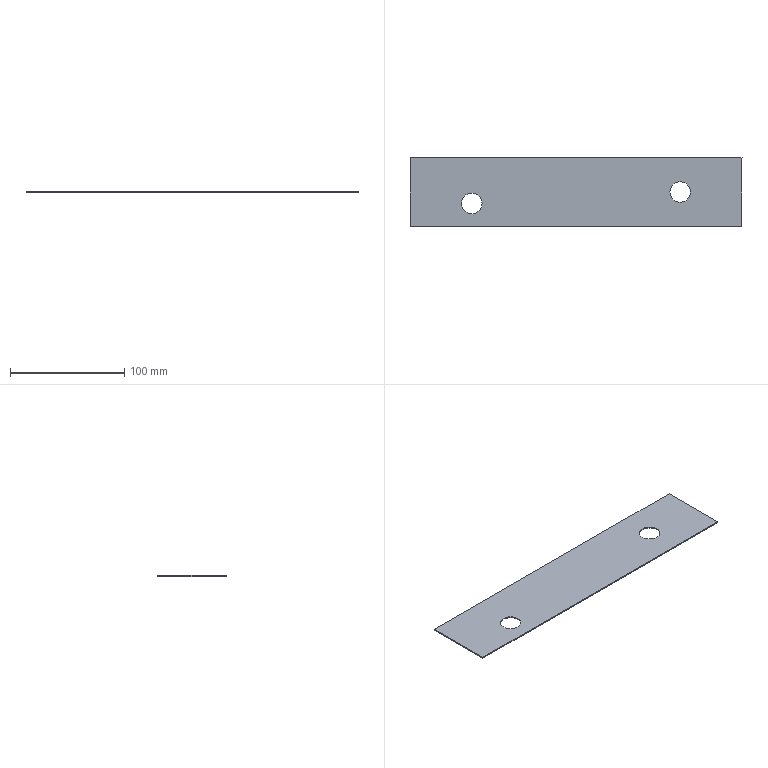Part | STEP file | lll_id506_x_t | 1 solid | 8 faces | box 290 x 60 x 1 mm | volume 16891 mm3 | plane 6 | cylinder 2 | commonest cylinder face diameters 18.009 x2
STEP:
#1=CARTESIAN_POINT('',(2237.435,600.,222.5));
#2=VERTEX_POINT('',#1);
#3=CARTESIAN_POINT('',(2237.435,660.,222.5));
#4=VERTEX_POINT('',#3);
#5=CARTESIAN_POINT('',(2237.435,551.,222.5));
#6=DIRECTION('',(0.,1.,0.));
#7=VECTOR('',#6,1.);
#8=LINE('',#5,#7);
#9=EDGE_CURVE('',#2,#4,#8,.T.);
#10=ORIENTED_EDGE('',*,*,#9,.T.);
#11=CARTESIAN_POINT('',(2237.435,660.,223.5));
#12=VERTEX_POINT('',#11);
#13=CARTESIAN_POINT('',(2237.435,660.,223.5));
#14=DIRECTION('',(0.,0.,-1.));
#15=VECTOR('',#14,1.);
#16=LINE('',#13,#15);
#17=EDGE_CURVE('',#12,#4,#16,.T.);
#18=ORIENTED_EDGE('',*,*,#17,.F.);
#19=CARTESIAN_POINT('',(2237.435,600.,223.5));
#20=VERTEX_POINT('',#19);
#21=CARTESIAN_POINT('',(2237.435,551.,223.5));
#22=DIRECTION('',(0.,1.,0.));
#23=VECTOR('',#22,1.);
#24=LINE('',#21,#23);
#25=EDGE_CURVE('',#20,#12,#24,.T.);
#26=ORIENTED_EDGE('',*,*,#25,.F.);
#27=CARTESIAN_POINT('',(2237.435,600.,223.5));
#28=DIRECTION('',(0.,0.,-1.));
#29=VECTOR('',#28,1.);
#30=LINE('',#27,#29);
#31=EDGE_CURVE('',#20,#2,#30,.T.);
#32=ORIENTED_EDGE('',*,*,#31,.T.);
#33=EDGE_LOOP('',(#10,#18,#26,#32));
#34=FACE_OUTER_BOUND('',#33,.T.);
#35=CARTESIAN_POINT('',(2237.435,551.,223.5));
#36=DIRECTION('',(-1.,0.,0.));
#37=DIRECTION('',(0.,1.,0.));
#38=AXIS2_PLACEMENT_3D('',#35,#36,#37);
#39=PLANE('',#38);
#40=ADVANCED_FACE('',(#34),#39,.F.);
#41=CARTESIAN_POINT('',(1947.435,660.,222.5));
#42=VERTEX_POINT('',#41);
#43=CARTESIAN_POINT('',(2052.435,660.,222.5));
#44=DIRECTION('',(1.,0.,0.));
#45=VECTOR('',#44,1.);
#46=LINE('',#43,#45);
#47=EDGE_CURVE('',#42,#4,#46,.T.);
#48=ORIENTED_EDGE('',*,*,#47,.F.);
#49=CARTESIAN_POINT('',(1947.435,660.,223.5));
#50=VERTEX_POINT('',#49);
#51=CARTESIAN_POINT('',(1947.435,660.,223.5));
#52=DIRECTION('',(0.,0.,-1.));
#53=VECTOR('',#52,1.);
#54=LINE('',#51,#53);
#55=EDGE_CURVE('',#50,#42,#54,.T.);
#56=ORIENTED_EDGE('',*,*,#55,.F.);
#57=CARTESIAN_POINT('',(2052.435,660.,223.5));
#58=DIRECTION('',(1.,0.,0.));
#59=VECTOR('',#58,1.);
#60=LINE('',#57,#59);
#61=EDGE_CURVE('',#50,#12,#60,.T.);
#62=ORIENTED_EDGE('',*,*,#61,.T.);
#63=ORIENTED_EDGE('',*,*,#17,.T.);
#64=EDGE_LOOP('',(#48,#56,#62,#63));
#65=FACE_OUTER_BOUND('',#64,.T.);
#66=CARTESIAN_POINT('',(2052.435,660.,223.5));
#67=DIRECTION('',(0.,1.,0.));
#68=DIRECTION('',(1.,0.,0.));
#69=AXIS2_PLACEMENT_3D('',#66,#67,#68);
#70=PLANE('',#69);
#71=ADVANCED_FACE('',(#65),#70,.T.);
#72=CARTESIAN_POINT('',(1947.435,600.,222.5));
#73=VERTEX_POINT('',#72);
#74=CARTESIAN_POINT('',(1947.435,0.,222.5));
#75=DIRECTION('',(0.,1.,0.));
#76=VECTOR('',#75,1.);
#77=LINE('',#74,#76);
#78=EDGE_CURVE('',#73,#42,#77,.T.);
#79=ORIENTED_EDGE('',*,*,#78,.F.);
#80=CARTESIAN_POINT('',(1947.435,600.,223.5));
#81=VERTEX_POINT('',#80);
#82=CARTESIAN_POINT('',(1947.435,600.,223.5));
#83=DIRECTION('',(0.,0.,-1.));
#84=VECTOR('',#83,1.);
#85=LINE('',#82,#84);
#86=EDGE_CURVE('',#81,#73,#85,.T.);
#87=ORIENTED_EDGE('',*,*,#86,.F.);
#88=CARTESIAN_POINT('',(1947.435,0.,223.5));
#89=DIRECTION('',(0.,1.,0.));
#90=VECTOR('',#89,1.);
#91=LINE('',#88,#90);
#92=EDGE_CURVE('',#81,#50,#91,.T.);
#93=ORIENTED_EDGE('',*,*,#92,.T.);
#94=ORIENTED_EDGE('',*,*,#55,.T.);
#95=EDGE_LOOP('',(#79,#87,#93,#94));
#96=FACE_OUTER_BOUND('',#95,.T.);
#97=CARTESIAN_POINT('',(1947.435,0.,223.5));
#98=DIRECTION('',(-1.,0.,0.));
#99=DIRECTION('',(0.,1.,0.));
#100=AXIS2_PLACEMENT_3D('',#97,#98,#99);
#101=PLANE('',#100);
#102=ADVANCED_FACE('',(#96),#101,.T.);
#103=CARTESIAN_POINT('',(1992.431,620.,222.5));
#104=VERTEX_POINT('',#103);
#105=CARTESIAN_POINT('',(2001.435,620.,222.5));
#106=DIRECTION('',(0.,0.,-1.));
#107=DIRECTION('',(-1.,0.,0.));
#108=AXIS2_PLACEMENT_3D('',#105,#106,#107);
#109=CIRCLE('',#108,9.005);
#110=EDGE_CURVE('',#104,#104,#109,.T.);
#111=ORIENTED_EDGE('',*,*,#110,.T.);
#112=EDGE_LOOP('',(#111));
#113=FACE_BOUND('',#112,.T.);
#114=CARTESIAN_POINT('',(1992.431,620.,223.5));
#115=VERTEX_POINT('',#114);
#116=CARTESIAN_POINT('',(2001.435,620.,223.5));
#117=DIRECTION('',(0.,0.,-1.));
#118=DIRECTION('',(-1.,0.,0.));
#119=AXIS2_PLACEMENT_3D('',#116,#117,#118);
#120=CIRCLE('',#119,9.005);
#121=EDGE_CURVE('',#115,#115,#120,.T.);
#122=ORIENTED_EDGE('',*,*,#121,.F.);
#123=EDGE_LOOP('',(#122));
#124=FACE_BOUND('',#123,.T.);
#125=CARTESIAN_POINT('',(2001.435,620.,223.5));
#126=DIRECTION('',(0.,0.,-1.));
#127=DIRECTION('',(1.,0.,0.));
#128=AXIS2_PLACEMENT_3D('',#125,#126,#127);
#129=CYLINDRICAL_SURFACE('',#128,9.005);
#130=ADVANCED_FACE('',(#113,#124),#129,.F.);
#131=CARTESIAN_POINT('',(2174.431,630.,222.5));
#132=VERTEX_POINT('',#131);
#133=CARTESIAN_POINT('',(2183.435,630.,222.5));
#134=DIRECTION('',(0.,0.,-1.));
#135=DIRECTION('',(-1.,0.,0.));
#136=AXIS2_PLACEMENT_3D('',#133,#134,#135);
#137=CIRCLE('',#136,9.005);
#138=EDGE_CURVE('',#132,#132,#137,.T.);
#139=ORIENTED_EDGE('',*,*,#138,.T.);
#140=EDGE_LOOP('',(#139));
#141=FACE_BOUND('',#140,.T.);
#142=CARTESIAN_POINT('',(2174.431,630.,223.5));
#143=VERTEX_POINT('',#142);
#144=CARTESIAN_POINT('',(2183.435,630.,223.5));
#145=DIRECTION('',(0.,0.,-1.));
#146=DIRECTION('',(-1.,0.,0.));
#147=AXIS2_PLACEMENT_3D('',#144,#145,#146);
#148=CIRCLE('',#147,9.005);
#149=EDGE_CURVE('',#143,#143,#148,.T.);
#150=ORIENTED_EDGE('',*,*,#149,.F.);
#151=EDGE_LOOP('',(#150));
#152=FACE_BOUND('',#151,.T.);
#153=CARTESIAN_POINT('',(2183.435,630.,223.5));
#154=DIRECTION('',(0.,0.,-1.));
#155=DIRECTION('',(1.,0.,0.));
#156=AXIS2_PLACEMENT_3D('',#153,#154,#155);
#157=CYLINDRICAL_SURFACE('',#156,9.005);
#158=ADVANCED_FACE('',(#141,#152),#157,.F.);
#159=CARTESIAN_POINT('',(2052.435,600.,222.5));
#160=DIRECTION('',(1.,0.,0.));
#161=VECTOR('',#160,1.);
#162=LINE('',#159,#161);
#163=EDGE_CURVE('',#73,#2,#162,.T.);
#164=ORIENTED_EDGE('',*,*,#163,.T.);
#165=ORIENTED_EDGE('',*,*,#31,.F.);
#166=CARTESIAN_POINT('',(2052.435,600.,223.5));
#167=DIRECTION('',(1.,0.,0.));
#168=VECTOR('',#167,1.);
#169=LINE('',#166,#168);
#170=EDGE_CURVE('',#81,#20,#169,.T.);
#171=ORIENTED_EDGE('',*,*,#170,.F.);
#172=ORIENTED_EDGE('',*,*,#86,.T.);
#173=EDGE_LOOP('',(#164,#165,#171,#172));
#174=FACE_OUTER_BOUND('',#173,.T.);
#175=CARTESIAN_POINT('',(2052.435,600.,223.5));
#176=DIRECTION('',(0.,1.,0.));
#177=DIRECTION('',(0.,0.,-1.));
#178=AXIS2_PLACEMENT_3D('',#175,#176,#177);
#179=PLANE('',#178);
#180=ADVANCED_FACE('',(#174),#179,.F.);
#181=ORIENTED_EDGE('',*,*,#149,.T.);
#182=EDGE_LOOP('',(#181));
#183=FACE_BOUND('',#182,.T.);
#184=ORIENTED_EDGE('',*,*,#121,.T.);
#185=EDGE_LOOP('',(#184));
#186=FACE_BOUND('',#185,.T.);
#187=ORIENTED_EDGE('',*,*,#25,.T.);
#188=ORIENTED_EDGE('',*,*,#61,.F.);
#189=ORIENTED_EDGE('',*,*,#92,.F.);
#190=ORIENTED_EDGE('',*,*,#170,.T.);
#191=EDGE_LOOP('',(#187,#188,#189,#190));
#192=FACE_BOUND('',#191,.T.);
#193=CARTESIAN_POINT('',(2052.435,0.,223.5));
#194=DIRECTION('',(0.,0.,1.));
#195=DIRECTION('',(-1.,0.,0.));
#196=AXIS2_PLACEMENT_3D('',#193,#194,#195);
#197=PLANE('',#196);
#198=ADVANCED_FACE('',(#183,#186,#192),#197,.T.);
#199=ORIENTED_EDGE('',*,*,#138,.F.);
#200=EDGE_LOOP('',(#199));
#201=FACE_BOUND('',#200,.T.);
#202=ORIENTED_EDGE('',*,*,#110,.F.);
#203=EDGE_LOOP('',(#202));
#204=FACE_BOUND('',#203,.T.);
#205=ORIENTED_EDGE('',*,*,#9,.F.);
#206=ORIENTED_EDGE('',*,*,#163,.F.);
#207=ORIENTED_EDGE('',*,*,#78,.T.);
#208=ORIENTED_EDGE('',*,*,#47,.T.);
#209=EDGE_LOOP('',(#205,#206,#207,#208));
#210=FACE_BOUND('',#209,.T.);
#211=CARTESIAN_POINT('',(2052.435,0.,222.5));
#212=DIRECTION('',(0.,0.,1.));
#213=DIRECTION('',(-1.,0.,0.));
#214=AXIS2_PLACEMENT_3D('',#211,#212,#213);
#215=PLANE('',#214);
#216=ADVANCED_FACE('',(#201,#204,#210),#215,.F.);
#217=CLOSED_SHELL('',(#40,#71,#102,#130,#158,#180,#198,#216));
#218=MANIFOLD_SOLID_BREP('',#217);
#219=(LENGTH_UNIT()NAMED_UNIT(*)SI_UNIT(.MILLI.,.METRE.));
#220=UNCERTAINTY_MEASURE_WITH_UNIT(LENGTH_MEASURE(0.00002),#219,'','');
#221=(NAMED_UNIT(*)PLANE_ANGLE_UNIT()SI_UNIT($,.RADIAN.));
#222=PLANE_ANGLE_MEASURE_WITH_UNIT(PLANE_ANGLE_MEASURE(0.01745),#221);
#223=DIMENSIONAL_EXPONENTS(0.,0.,0.,0.,0.,0.,0.);
#224=(CONVERSION_BASED_UNIT('DEGREE',#222)NAMED_UNIT(#223)PLANE_ANGLE_UNIT());
#225=(NAMED_UNIT(*)SI_UNIT($,.STERADIAN.)SOLID_ANGLE_UNIT());
#226=(GEOMETRIC_REPRESENTATION_CONTEXT(3)GLOBAL_UNCERTAINTY_ASSIGNED_CONTEXT((#220))GLOBAL_UNIT_ASSIGNED_CONTEXT((#219,#224,#225))REPRESENTATION_CONTEXT('',''));
#227=ADVANCED_BREP_SHAPE_REPRESENTATION('',(#218),#226);